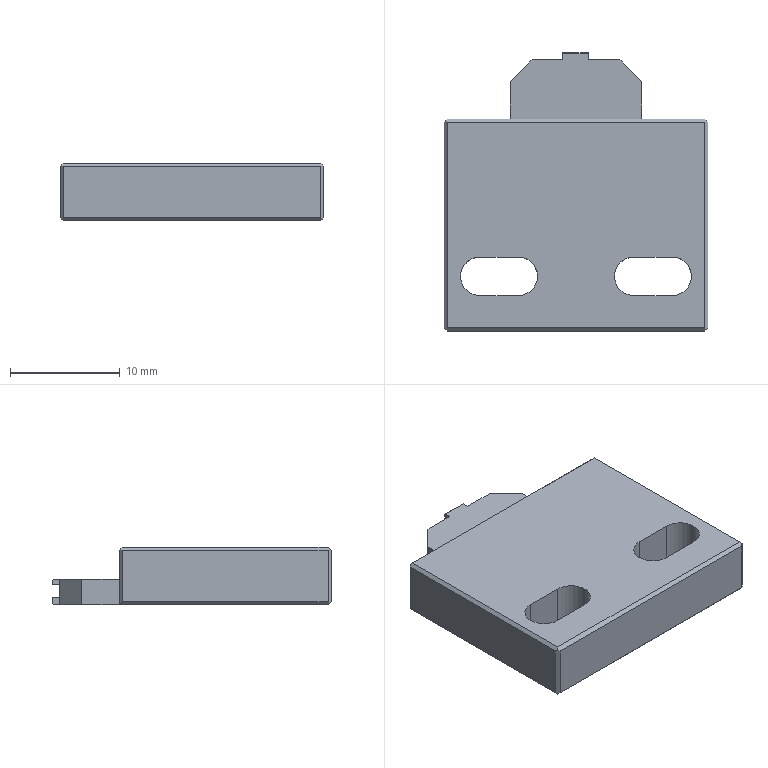Part | NX | 1 solid | 43 faces | box 24 x 25.342 x 5.25 mm | volume 2337 mm3 | plane 37 | cylinder 6 | commonest cylinder face diameters 3.5 x6
STEP:
#1=CARTESIAN_POINT('',(-1.2,-32.158,5.225));
#2=VERTEX_POINT('',#1);
#3=CARTESIAN_POINT('',(1.1,-32.158,5.225));
#4=VERTEX_POINT('',#3);
#5=CARTESIAN_POINT('',(-0.05,-32.158,5.225));
#6=DIRECTION('',(1.,0.,0.));
#7=VECTOR('',#6,1000.);
#8=LINE('',#5,#7);
#9=EDGE_CURVE('',#2,#4,#8,.T.);
#10=ORIENTED_EDGE('',*,*,#9,.T.);
#11=CARTESIAN_POINT('',(1.1,-32.158,4.822));
#12=VERTEX_POINT('',#11);
#13=CARTESIAN_POINT('',(1.1,-32.158,0.));
#14=DIRECTION('',(0.,0.,1.));
#15=VECTOR('',#14,1000.);
#16=LINE('',#13,#15);
#17=EDGE_CURVE('',#12,#4,#16,.T.);
#18=ORIENTED_EDGE('',*,*,#17,.F.);
#19=CARTESIAN_POINT('',(-1.2,-32.158,4.822));
#20=VERTEX_POINT('',#19);
#21=CARTESIAN_POINT('',(0.,-32.158,4.822));
#22=DIRECTION('',(-1.,0.,0.));
#23=VECTOR('',#22,1000.);
#24=LINE('',#21,#23);
#25=EDGE_CURVE('',#12,#20,#24,.T.);
#26=ORIENTED_EDGE('',*,*,#25,.T.);
#27=CARTESIAN_POINT('',(-1.2,-32.158,0.));
#28=DIRECTION('',(0.,0.,-1.));
#29=VECTOR('',#28,1000.);
#30=LINE('',#27,#29);
#31=EDGE_CURVE('',#2,#20,#30,.T.);
#32=ORIENTED_EDGE('',*,*,#31,.F.);
#33=EDGE_LOOP('',(#10,#18,#26,#32));
#34=FACE_BOUND('',#33,.T.);
#35=CARTESIAN_POINT('',(-4.2,-32.158,8.775));
#36=DIRECTION('',(0.,-1.,0.));
#37=DIRECTION('',(-1.,0.,0.));
#38=AXIS2_PLACEMENT_3D('',#35,#36,#37);
#39=PLANE('',#38);
#40=ADVANCED_FACE('',(#34),#39,.F.);
#41=ORIENTED_EDGE('',*,*,#9,.F.);
#42=CARTESIAN_POINT('',(-1.2,-32.258,5.325));
#43=VERTEX_POINT('',#42);
#44=CARTESIAN_POINT('',(-1.2,0.,-26.933));
#45=DIRECTION('',(0.,0.7071,-0.7071));
#46=VECTOR('',#45,1000.);
#47=LINE('',#44,#46);
#48=EDGE_CURVE('',#43,#2,#47,.T.);
#49=ORIENTED_EDGE('',*,*,#48,.F.);
#50=CARTESIAN_POINT('',(1.1,-32.258,5.325));
#51=VERTEX_POINT('',#50);
#52=CARTESIAN_POINT('',(-0.05,-32.258,5.325));
#53=DIRECTION('',(1.,0.,0.));
#54=VECTOR('',#53,1000.);
#55=LINE('',#52,#54);
#56=EDGE_CURVE('',#43,#51,#55,.T.);
#57=ORIENTED_EDGE('',*,*,#56,.T.);
#58=CARTESIAN_POINT('',(1.1,0.,-26.933));
#59=DIRECTION('',(0.,-0.7071,0.7071));
#60=VECTOR('',#59,1000.);
#61=LINE('',#58,#60);
#62=EDGE_CURVE('',#4,#51,#61,.T.);
#63=ORIENTED_EDGE('',*,*,#62,.F.);
#64=EDGE_LOOP('',(#41,#49,#57,#63));
#65=FACE_BOUND('',#64,.T.);
#66=CARTESIAN_POINT('',(-0.05,-32.208,5.275));
#67=DIRECTION('',(0.,0.7071,0.7071));
#68=DIRECTION('',(1.,0.,0.));
#69=AXIS2_PLACEMENT_3D('',#66,#67,#68);
#70=PLANE('',#69);
#71=ADVANCED_FACE('',(#65),#70,.T.);
#72=CARTESIAN_POINT('',(1.1,-32.158,3.1));
#73=VERTEX_POINT('',#72);
#74=CARTESIAN_POINT('',(-1.2,-32.158,3.1));
#75=VERTEX_POINT('',#74);
#76=CARTESIAN_POINT('',(-0.05,-32.158,3.1));
#77=DIRECTION('',(-1.,0.,0.));
#78=VECTOR('',#77,1000.);
#79=LINE('',#76,#78);
#80=EDGE_CURVE('',#73,#75,#79,.T.);
#81=ORIENTED_EDGE('',*,*,#80,.T.);
#82=CARTESIAN_POINT('',(-1.2,-32.158,3.7));
#83=VERTEX_POINT('',#82);
#84=CARTESIAN_POINT('',(-1.2,-32.158,0.));
#85=DIRECTION('',(0.,0.,-1.));
#86=VECTOR('',#85,1000.);
#87=LINE('',#84,#86);
#88=EDGE_CURVE('',#83,#75,#87,.T.);
#89=ORIENTED_EDGE('',*,*,#88,.F.);
#90=CARTESIAN_POINT('',(1.1,-32.158,3.7));
#91=VERTEX_POINT('',#90);
#92=CARTESIAN_POINT('',(0.,-32.158,3.7));
#93=DIRECTION('',(1.,0.,0.));
#94=VECTOR('',#93,1000.);
#95=LINE('',#92,#94);
#96=EDGE_CURVE('',#83,#91,#95,.T.);
#97=ORIENTED_EDGE('',*,*,#96,.T.);
#98=CARTESIAN_POINT('',(1.1,-32.158,0.));
#99=DIRECTION('',(0.,0.,1.));
#100=VECTOR('',#99,1000.);
#101=LINE('',#98,#100);
#102=EDGE_CURVE('',#73,#91,#101,.T.);
#103=ORIENTED_EDGE('',*,*,#102,.F.);
#104=EDGE_LOOP('',(#81,#89,#97,#103));
#105=FACE_BOUND('',#104,.T.);
#106=CARTESIAN_POINT('',(0.,-32.158,4.111));
#107=DIRECTION('',(0.,1.,0.));
#108=DIRECTION('',(1.,0.,0.));
#109=AXIS2_PLACEMENT_3D('',#106,#107,#108);
#110=PLANE('',#109);
#111=ADVANCED_FACE('',(#105),#110,.T.);
#112=ORIENTED_EDGE('',*,*,#80,.F.);
#113=CARTESIAN_POINT('',(1.1,-32.258,3.));
#114=VERTEX_POINT('',#113);
#115=CARTESIAN_POINT('',(1.1,0.,35.258));
#116=DIRECTION('',(0.,0.7071,0.7071));
#117=VECTOR('',#116,1000.);
#118=LINE('',#115,#117);
#119=EDGE_CURVE('',#114,#73,#118,.T.);
#120=ORIENTED_EDGE('',*,*,#119,.F.);
#121=CARTESIAN_POINT('',(-1.2,-32.258,3.));
#122=VERTEX_POINT('',#121);
#123=CARTESIAN_POINT('',(-0.05,-32.258,3.));
#124=DIRECTION('',(-1.,0.,0.));
#125=VECTOR('',#124,1000.);
#126=LINE('',#123,#125);
#127=EDGE_CURVE('',#114,#122,#126,.T.);
#128=ORIENTED_EDGE('',*,*,#127,.T.);
#129=CARTESIAN_POINT('',(-1.2,0.,35.258));
#130=DIRECTION('',(0.,-0.7071,-0.7071));
#131=VECTOR('',#130,1000.);
#132=LINE('',#129,#131);
#133=EDGE_CURVE('',#75,#122,#132,.T.);
#134=ORIENTED_EDGE('',*,*,#133,.F.);
#135=EDGE_LOOP('',(#112,#120,#128,#134));
#136=FACE_BOUND('',#135,.T.);
#137=CARTESIAN_POINT('',(-0.05,-32.208,3.05));
#138=DIRECTION('',(0.,0.7071,-0.7071));
#139=DIRECTION('',(-1.,0.,0.));
#140=AXIS2_PLACEMENT_3D('',#137,#138,#139);
#141=PLANE('',#140);
#142=ADVANCED_FACE('',(#136),#141,.T.);
#143=ORIENTED_EDGE('',*,*,#102,.T.);
#144=CARTESIAN_POINT('',(1.1,-32.815,3.7));
#145=VERTEX_POINT('',#144);
#146=CARTESIAN_POINT('',(1.1,0.,3.7));
#147=DIRECTION('',(0.,-1.,0.));
#148=VECTOR('',#147,1000.);
#149=LINE('',#146,#148);
#150=EDGE_CURVE('',#91,#145,#149,.T.);
#151=ORIENTED_EDGE('',*,*,#150,.T.);
#152=CARTESIAN_POINT('',(1.1,-32.815,3.));
#153=VERTEX_POINT('',#152);
#154=CARTESIAN_POINT('',(1.1,-32.815,0.));
#155=DIRECTION('',(0.,0.,1.));
#156=VECTOR('',#155,1000.);
#157=LINE('',#154,#156);
#158=EDGE_CURVE('',#153,#145,#157,.T.);
#159=ORIENTED_EDGE('',*,*,#158,.F.);
#160=CARTESIAN_POINT('',(1.1,0.,3.));
#161=DIRECTION('',(0.,1.,0.));
#162=VECTOR('',#161,1000.);
#163=LINE('',#160,#162);
#164=EDGE_CURVE('',#153,#114,#163,.T.);
#165=ORIENTED_EDGE('',*,*,#164,.T.);
#166=ORIENTED_EDGE('',*,*,#119,.T.);
#167=EDGE_LOOP('',(#143,#151,#159,#165,#166));
#168=FACE_BOUND('',#167,.T.);
#169=CARTESIAN_POINT('',(1.1,-33.565,2.475));
#170=DIRECTION('',(-1.,0.,0.));
#171=DIRECTION('',(0.,0.,1.));
#172=AXIS2_PLACEMENT_3D('',#169,#170,#171);
#173=PLANE('',#172);
#174=ADVANCED_FACE('',(#168),#173,.F.);
#175=ORIENTED_EDGE('',*,*,#150,.F.);
#176=ORIENTED_EDGE('',*,*,#96,.F.);
#177=CARTESIAN_POINT('',(-1.2,-32.815,3.7));
#178=VERTEX_POINT('',#177);
#179=CARTESIAN_POINT('',(-1.2,0.,3.7));
#180=DIRECTION('',(0.,1.,0.));
#181=VECTOR('',#180,1000.);
#182=LINE('',#179,#181);
#183=EDGE_CURVE('',#178,#83,#182,.T.);
#184=ORIENTED_EDGE('',*,*,#183,.F.);
#185=CARTESIAN_POINT('',(0.,-32.815,3.7));
#186=DIRECTION('',(-1.,0.,0.));
#187=VECTOR('',#186,1000.);
#188=LINE('',#185,#187);
#189=EDGE_CURVE('',#145,#178,#188,.T.);
#190=ORIENTED_EDGE('',*,*,#189,.F.);
#191=EDGE_LOOP('',(#175,#176,#184,#190));
#192=FACE_BOUND('',#191,.T.);
#193=CARTESIAN_POINT('',(6.,-34.,3.7));
#194=DIRECTION('',(0.,0.,1.));
#195=DIRECTION('',(0.,-1.,0.));
#196=AXIS2_PLACEMENT_3D('',#193,#194,#195);
#197=PLANE('',#196);
#198=ADVANCED_FACE('',(#192),#197,.T.);
#199=CARTESIAN_POINT('',(-4.,-32.815,5.325));
#200=VERTEX_POINT('',#199);
#201=CARTESIAN_POINT('',(-4.,-32.815,3.));
#202=VERTEX_POINT('',#201);
#203=CARTESIAN_POINT('',(-4.,-32.815,4.175));
#204=DIRECTION('',(0.,0.,-1.));
#205=VECTOR('',#204,1000.);
#206=LINE('',#203,#205);
#207=EDGE_CURVE('',#200,#202,#206,.T.);
#208=ORIENTED_EDGE('',*,*,#207,.F.);
#209=CARTESIAN_POINT('',(-1.2,-32.815,5.325));
#210=VERTEX_POINT('',#209);
#211=CARTESIAN_POINT('',(0.,-32.815,5.325));
#212=DIRECTION('',(1.,0.,0.));
#213=VECTOR('',#212,1000.);
#214=LINE('',#211,#213);
#215=EDGE_CURVE('',#200,#210,#214,.T.);
#216=ORIENTED_EDGE('',*,*,#215,.T.);
#217=CARTESIAN_POINT('',(-1.2,-32.815,4.822));
#218=VERTEX_POINT('',#217);
#219=CARTESIAN_POINT('',(-1.2,-32.815,0.));
#220=DIRECTION('',(0.,0.,-1.));
#221=VECTOR('',#220,1000.);
#222=LINE('',#219,#221);
#223=EDGE_CURVE('',#210,#218,#222,.T.);
#224=ORIENTED_EDGE('',*,*,#223,.T.);
#225=CARTESIAN_POINT('',(1.1,-32.815,4.822));
#226=VERTEX_POINT('',#225);
#227=CARTESIAN_POINT('',(0.,-32.815,4.822));
#228=DIRECTION('',(1.,0.,0.));
#229=VECTOR('',#228,1000.);
#230=LINE('',#227,#229);
#231=EDGE_CURVE('',#218,#226,#230,.T.);
#232=ORIENTED_EDGE('',*,*,#231,.T.);
#233=CARTESIAN_POINT('',(1.1,-32.815,5.325));
#234=VERTEX_POINT('',#233);
#235=CARTESIAN_POINT('',(1.1,-32.815,0.));
#236=DIRECTION('',(0.,0.,-1.));
#237=VECTOR('',#236,1000.);
#238=LINE('',#235,#237);
#239=EDGE_CURVE('',#234,#226,#238,.T.);
#240=ORIENTED_EDGE('',*,*,#239,.F.);
#241=CARTESIAN_POINT('',(4.,-32.815,5.325));
#242=VERTEX_POINT('',#241);
#243=CARTESIAN_POINT('',(0.,-32.815,5.325));
#244=DIRECTION('',(1.,0.,0.));
#245=VECTOR('',#244,1000.);
#246=LINE('',#243,#245);
#247=EDGE_CURVE('',#234,#242,#246,.T.);
#248=ORIENTED_EDGE('',*,*,#247,.T.);
#249=CARTESIAN_POINT('',(4.,-32.815,3.));
#250=VERTEX_POINT('',#249);
#251=CARTESIAN_POINT('',(4.,-32.815,4.175));
#252=DIRECTION('',(0.,0.,1.));
#253=VECTOR('',#252,1000.);
#254=LINE('',#251,#253);
#255=EDGE_CURVE('',#250,#242,#254,.T.);
#256=ORIENTED_EDGE('',*,*,#255,.F.);
#257=CARTESIAN_POINT('',(0.,-32.815,3.));
#258=DIRECTION('',(-1.,0.,0.));
#259=VECTOR('',#258,1000.);
#260=LINE('',#257,#259);
#261=EDGE_CURVE('',#250,#153,#260,.T.);
#262=ORIENTED_EDGE('',*,*,#261,.T.);
#263=ORIENTED_EDGE('',*,*,#158,.T.);
#264=ORIENTED_EDGE('',*,*,#189,.T.);
#265=CARTESIAN_POINT('',(-1.2,-32.815,3.));
#266=VERTEX_POINT('',#265);
#267=CARTESIAN_POINT('',(-1.2,-32.815,0.));
#268=DIRECTION('',(0.,0.,-1.));
#269=VECTOR('',#268,1000.);
#270=LINE('',#267,#269);
#271=EDGE_CURVE('',#178,#266,#270,.T.);
#272=ORIENTED_EDGE('',*,*,#271,.T.);
#273=CARTESIAN_POINT('',(0.,-32.815,3.));
#274=DIRECTION('',(-1.,0.,0.));
#275=VECTOR('',#274,1000.);
#276=LINE('',#273,#275);
#277=EDGE_CURVE('',#266,#202,#276,.T.);
#278=ORIENTED_EDGE('',*,*,#277,.T.);
#279=EDGE_LOOP('',(#208,#216,#224,#232,#240,#248,#256,#262,#263,#264,#272,#278));
#280=FACE_BOUND('',#279,.T.);
#281=CARTESIAN_POINT('',(6.,-32.815,2.475));
#282=DIRECTION('',(0.,-1.,0.));
#283=DIRECTION('',(0.,0.,-1.));
#284=AXIS2_PLACEMENT_3D('',#281,#282,#283);
#285=PLANE('',#284);
#286=ADVANCED_FACE('',(#280),#285,.F.);
#287=CARTESIAN_POINT('',(11.7,-38.2,3.));
#288=VERTEX_POINT('',#287);
#289=CARTESIAN_POINT('',(11.7,-57.2,3.));
#290=VERTEX_POINT('',#289);
#291=CARTESIAN_POINT('',(11.7,-47.85,3.));
#292=DIRECTION('',(0.,-1.,0.));
#293=VECTOR('',#292,1000.);
#294=LINE('',#291,#293);
#295=EDGE_CURVE('',#288,#290,#294,.T.);
#296=ORIENTED_EDGE('',*,*,#295,.T.);
#297=CARTESIAN_POINT('',(-11.7,-57.2,3.));
#298=VERTEX_POINT('',#297);
#299=CARTESIAN_POINT('',(0.,-57.2,3.));
#300=DIRECTION('',(1.,0.,0.));
#301=VECTOR('',#300,1000.);
#302=LINE('',#299,#301);
#303=EDGE_CURVE('',#298,#290,#302,.T.);
#304=ORIENTED_EDGE('',*,*,#303,.F.);
#305=CARTESIAN_POINT('',(-11.7,-38.2,3.));
#306=VERTEX_POINT('',#305);
#307=CARTESIAN_POINT('',(-11.7,-47.85,3.));
#308=DIRECTION('',(0.,-1.,0.));
#309=VECTOR('',#308,1000.);
#310=LINE('',#307,#309);
#311=EDGE_CURVE('',#306,#298,#310,.T.);
#312=ORIENTED_EDGE('',*,*,#311,.F.);
#313=CARTESIAN_POINT('',(-6.,-38.2,3.));
#314=VERTEX_POINT('',#313);
#315=CARTESIAN_POINT('',(0.,-38.2,3.));
#316=DIRECTION('',(-1.,0.,0.));
#317=VECTOR('',#316,1000.);
#318=LINE('',#315,#317);
#319=EDGE_CURVE('',#314,#306,#318,.T.);
#320=ORIENTED_EDGE('',*,*,#319,.F.);
#321=CARTESIAN_POINT('',(-6.,-34.815,3.));
#322=VERTEX_POINT('',#321);
#323=CARTESIAN_POINT('',(-6.,-33.565,3.));
#324=DIRECTION('',(0.,1.,0.));
#325=VECTOR('',#324,1000.);
#326=LINE('',#323,#325);
#327=EDGE_CURVE('',#314,#322,#326,.T.);
#328=ORIENTED_EDGE('',*,*,#327,.T.);
#329=CARTESIAN_POINT('',(28.815,0.,3.));
#330=DIRECTION('',(0.7071,0.7071,0.));
#331=VECTOR('',#330,1000.);
#332=LINE('',#329,#331);
#333=EDGE_CURVE('',#322,#202,#332,.T.);
#334=ORIENTED_EDGE('',*,*,#333,.T.);
#335=ORIENTED_EDGE('',*,*,#277,.F.);
#336=CARTESIAN_POINT('',(-1.2,0.,3.));
#337=DIRECTION('',(0.,-1.,0.));
#338=VECTOR('',#337,1000.);
#339=LINE('',#336,#338);
#340=EDGE_CURVE('',#122,#266,#339,.T.);
#341=ORIENTED_EDGE('',*,*,#340,.F.);
#342=ORIENTED_EDGE('',*,*,#127,.F.);
#343=ORIENTED_EDGE('',*,*,#164,.F.);
#344=ORIENTED_EDGE('',*,*,#261,.F.);
#345=CARTESIAN_POINT('',(6.,-34.815,3.));
#346=VERTEX_POINT('',#345);
#347=CARTESIAN_POINT('',(-28.815,0.,3.));
#348=DIRECTION('',(-0.7071,0.7071,0.));
#349=VECTOR('',#348,1000.);
#350=LINE('',#347,#349);
#351=EDGE_CURVE('',#346,#250,#350,.T.);
#352=ORIENTED_EDGE('',*,*,#351,.F.);
#353=CARTESIAN_POINT('',(6.,-38.2,3.));
#354=VERTEX_POINT('',#353);
#355=CARTESIAN_POINT('',(6.,0.,3.));
#356=DIRECTION('',(0.,1.,0.));
#357=VECTOR('',#356,1000.);
#358=LINE('',#355,#357);
#359=EDGE_CURVE('',#354,#346,#358,.T.);
#360=ORIENTED_EDGE('',*,*,#359,.F.);
#361=CARTESIAN_POINT('',(0.,-38.2,3.));
#362=DIRECTION('',(-1.,0.,0.));
#363=VECTOR('',#362,1000.);
#364=LINE('',#361,#363);
#365=EDGE_CURVE('',#288,#354,#364,.T.);
#366=ORIENTED_EDGE('',*,*,#365,.F.);
#367=EDGE_LOOP('',(#296,#304,#312,#320,#328,#334,#335,#341,#342,#343,#344,#352,#360,#366));
#368=FACE_BOUND('',#367,.T.);
#369=CARTESIAN_POINT('',(-5.25,-54.25,3.));
#370=VERTEX_POINT('',#369);
#371=CARTESIAN_POINT('',(-8.75,-54.25,3.));
#372=VERTEX_POINT('',#371);
#373=CARTESIAN_POINT('',(0.,-54.25,3.));
#374=DIRECTION('',(-1.,0.,0.));
#375=VECTOR('',#374,1000.);
#376=LINE('',#373,#375);
#377=EDGE_CURVE('',#370,#372,#376,.T.);
#378=ORIENTED_EDGE('',*,*,#377,.F.);
#379=CARTESIAN_POINT('',(-3.5,-52.5,3.));
#380=VERTEX_POINT('',#379);
#381=CARTESIAN_POINT('',(-5.25,-52.5,3.));
#382=DIRECTION('',(0.,0.,1.));
#383=DIRECTION('',(1.,0.,0.));
#384=AXIS2_PLACEMENT_3D('',#381,#382,#383);
#385=CIRCLE('',#384,1.75);
#386=EDGE_CURVE('',#370,#380,#385,.T.);
#387=ORIENTED_EDGE('',*,*,#386,.T.);
#388=CARTESIAN_POINT('',(-5.25,-50.75,3.));
#389=VERTEX_POINT('',#388);
#390=CARTESIAN_POINT('',(-5.25,-52.5,3.));
#391=DIRECTION('',(0.,0.,1.));
#392=DIRECTION('',(1.,0.,0.));
#393=AXIS2_PLACEMENT_3D('',#390,#391,#392);
#394=CIRCLE('',#393,1.75);
#395=EDGE_CURVE('',#380,#389,#394,.T.);
#396=ORIENTED_EDGE('',*,*,#395,.T.);
#397=CARTESIAN_POINT('',(-8.75,-50.75,3.));
#398=VERTEX_POINT('',#397);
#399=CARTESIAN_POINT('',(0.,-50.75,3.));
#400=DIRECTION('',(1.,0.,0.));
#401=VECTOR('',#400,1000.);
#402=LINE('',#399,#401);
#403=EDGE_CURVE('',#398,#389,#402,.T.);
#404=ORIENTED_EDGE('',*,*,#403,.F.);
#405=CARTESIAN_POINT('',(-8.75,-52.5,3.));
#406=DIRECTION('',(0.,0.,1.));
#407=DIRECTION('',(1.,0.,0.));
#408=AXIS2_PLACEMENT_3D('',#405,#406,#407);
#409=CIRCLE('',#408,1.75);
#410=EDGE_CURVE('',#398,#372,#409,.T.);
#411=ORIENTED_EDGE('',*,*,#410,.T.);
#412=EDGE_LOOP('',(#378,#387,#396,#404,#411));
#413=FACE_BOUND('',#412,.T.);
#414=CARTESIAN_POINT('',(8.75,-54.25,3.));
#415=VERTEX_POINT('',#414);
#416=CARTESIAN_POINT('',(5.25,-54.25,3.));
#417=VERTEX_POINT('',#416);
#418=CARTESIAN_POINT('',(0.,-54.25,3.));
#419=DIRECTION('',(-1.,0.,0.));
#420=VECTOR('',#419,1000.);
#421=LINE('',#418,#420);
#422=EDGE_CURVE('',#415,#417,#421,.T.);
#423=ORIENTED_EDGE('',*,*,#422,.F.);
#424=CARTESIAN_POINT('',(10.5,-52.5,3.));
#425=VERTEX_POINT('',#424);
#426=CARTESIAN_POINT('',(8.75,-52.5,3.));
#427=DIRECTION('',(0.,0.,1.));
#428=DIRECTION('',(1.,0.,0.));
#429=AXIS2_PLACEMENT_3D('',#426,#427,#428);
#430=CIRCLE('',#429,1.75);
#431=EDGE_CURVE('',#415,#425,#430,.T.);
#432=ORIENTED_EDGE('',*,*,#431,.T.);
#433=CARTESIAN_POINT('',(8.75,-50.75,3.));
#434=VERTEX_POINT('',#433);
#435=CARTESIAN_POINT('',(8.75,-52.5,3.));
#436=DIRECTION('',(0.,0.,1.));
#437=DIRECTION('',(1.,0.,0.));
#438=AXIS2_PLACEMENT_3D('',#435,#436,#437);
#439=CIRCLE('',#438,1.75);
#440=EDGE_CURVE('',#425,#434,#439,.T.);
#441=ORIENTED_EDGE('',*,*,#440,.T.);
#442=CARTESIAN_POINT('',(5.25,-50.75,3.));
#443=VERTEX_POINT('',#442);
#444=CARTESIAN_POINT('',(0.,-50.75,3.));
#445=DIRECTION('',(1.,0.,0.));
#446=VECTOR('',#445,1000.);
#447=LINE('',#444,#446);
#448=EDGE_CURVE('',#443,#434,#447,.T.);
#449=ORIENTED_EDGE('',*,*,#448,.F.);
#450=CARTESIAN_POINT('',(5.25,-52.5,3.));
#451=DIRECTION('',(0.,0.,1.));
#452=DIRECTION('',(1.,0.,0.));
#453=AXIS2_PLACEMENT_3D('',#450,#451,#452);
#454=CIRCLE('',#453,1.75);
#455=EDGE_CURVE('',#443,#417,#454,.T.);
#456=ORIENTED_EDGE('',*,*,#455,.T.);
#457=EDGE_LOOP('',(#423,#432,#441,#449,#456));
#458=FACE_BOUND('',#457,.T.);
#459=CARTESIAN_POINT('',(1.4,-33.565,3.));
#460=DIRECTION('',(0.,0.,-1.));
#461=DIRECTION('',(-1.,0.,0.));
#462=AXIS2_PLACEMENT_3D('',#459,#460,#461);
#463=PLANE('',#462);
#464=ADVANCED_FACE('',(#368,#413,#458),#463,.T.);
#465=CARTESIAN_POINT('',(10.5,-52.5,8.25));
#466=VERTEX_POINT('',#465);
#467=CARTESIAN_POINT('',(10.5,-52.5,2.475));
#468=DIRECTION('',(0.,0.,1.));
#469=VECTOR('',#468,1000.);
#470=LINE('',#467,#469);
#471=EDGE_CURVE('',#425,#466,#470,.T.);
#472=ORIENTED_EDGE('',*,*,#471,.F.);
#473=ORIENTED_EDGE('',*,*,#431,.F.);
#474=CARTESIAN_POINT('',(8.75,-54.25,8.25));
#475=VERTEX_POINT('',#474);
#476=CARTESIAN_POINT('',(8.75,-54.25,2.475));
#477=DIRECTION('',(0.,0.,1.));
#478=VECTOR('',#477,1000.);
#479=LINE('',#476,#478);
#480=EDGE_CURVE('',#415,#475,#479,.T.);
#481=ORIENTED_EDGE('',*,*,#480,.T.);
#482=CARTESIAN_POINT('',(8.75,-52.5,8.25));
#483=DIRECTION('',(0.,0.,1.));
#484=DIRECTION('',(1.,0.,0.));
#485=AXIS2_PLACEMENT_3D('',#482,#483,#484);
#486=CIRCLE('',#485,1.75);
#487=EDGE_CURVE('',#475,#466,#486,.T.);
#488=ORIENTED_EDGE('',*,*,#487,.T.);
#489=EDGE_LOOP('',(#472,#473,#481,#488));
#490=FACE_BOUND('',#489,.T.);
#491=CARTESIAN_POINT('',(8.75,-52.5,2.475));
#492=DIRECTION('',(0.,0.,1.));
#493=DIRECTION('',(1.,0.,0.));
#494=AXIS2_PLACEMENT_3D('',#491,#492,#493);
#495=CYLINDRICAL_SURFACE('',#494,1.75);
#496=ADVANCED_FACE('',(#490),#495,.F.);
#497=CARTESIAN_POINT('',(8.75,-50.75,8.25));
#498=VERTEX_POINT('',#497);
#499=CARTESIAN_POINT('',(5.25,-50.75,8.25));
#500=VERTEX_POINT('',#499);
#501=CARTESIAN_POINT('',(0.,-50.75,8.25));
#502=DIRECTION('',(-1.,0.,0.));
#503=VECTOR('',#502,1000.);
#504=LINE('',#501,#503);
#505=EDGE_CURVE('',#498,#500,#504,.T.);
#506=ORIENTED_EDGE('',*,*,#505,.T.);
#507=CARTESIAN_POINT('',(5.25,-50.75,2.475));
#508=DIRECTION('',(0.,0.,1.));
#509=VECTOR('',#508,1000.);
#510=LINE('',#507,#509);
#511=EDGE_CURVE('',#443,#500,#510,.T.);
#512=ORIENTED_EDGE('',*,*,#511,.F.);
#513=ORIENTED_EDGE('',*,*,#448,.T.);
#514=CARTESIAN_POINT('',(8.75,-50.75,2.475));
#515=DIRECTION('',(0.,0.,1.));
#516=VECTOR('',#515,1000.);
#517=LINE('',#514,#516);
#518=EDGE_CURVE('',#434,#498,#517,.T.);
#519=ORIENTED_EDGE('',*,*,#518,.T.);
#520=EDGE_LOOP('',(#506,#512,#513,#519));
#521=FACE_BOUND('',#520,.T.);
#522=CARTESIAN_POINT('',(5.25,-50.75,2.475));
#523=DIRECTION('',(0.,1.,0.));
#524=DIRECTION('',(1.,0.,0.));
#525=AXIS2_PLACEMENT_3D('',#522,#523,#524);
#526=PLANE('',#525);
#527=ADVANCED_FACE('',(#521),#526,.F.);
#528=ORIENTED_EDGE('',*,*,#422,.T.);
#529=CARTESIAN_POINT('',(5.25,-54.25,8.25));
#530=VERTEX_POINT('',#529);
#531=CARTESIAN_POINT('',(5.25,-54.25,2.475));
#532=DIRECTION('',(0.,0.,1.));
#533=VECTOR('',#532,1000.);
#534=LINE('',#531,#533);
#535=EDGE_CURVE('',#417,#530,#534,.T.);
#536=ORIENTED_EDGE('',*,*,#535,.T.);
#537=CARTESIAN_POINT('',(0.,-54.25,8.25));
#538=DIRECTION('',(1.,0.,0.));
#539=VECTOR('',#538,1000.);
#540=LINE('',#537,#539);
#541=EDGE_CURVE('',#530,#475,#540,.T.);
#542=ORIENTED_EDGE('',*,*,#541,.T.);
#543=ORIENTED_EDGE('',*,*,#480,.F.);
#544=EDGE_LOOP('',(#528,#536,#542,#543));
#545=FACE_BOUND('',#544,.T.);
#546=CARTESIAN_POINT('',(8.75,-54.25,2.475));
#547=DIRECTION('',(0.,-1.,0.));
#548=DIRECTION('',(0.,0.,-1.));
#549=AXIS2_PLACEMENT_3D('',#546,#547,#548);
#550=PLANE('',#549);
#551=ADVANCED_FACE('',(#545),#550,.F.);
#552=ORIENTED_EDGE('',*,*,#455,.F.);
#553=ORIENTED_EDGE('',*,*,#511,.T.);
#554=CARTESIAN_POINT('',(5.25,-52.5,8.25));
#555=DIRECTION('',(0.,0.,1.));
#556=DIRECTION('',(1.,0.,0.));
#557=AXIS2_PLACEMENT_3D('',#554,#555,#556);
#558=CIRCLE('',#557,1.75);
#559=EDGE_CURVE('',#500,#530,#558,.T.);
#560=ORIENTED_EDGE('',*,*,#559,.T.);
#561=ORIENTED_EDGE('',*,*,#535,.F.);
#562=EDGE_LOOP('',(#552,#553,#560,#561));
#563=FACE_BOUND('',#562,.T.);
#564=CARTESIAN_POINT('',(5.25,-52.5,2.475));
#565=DIRECTION('',(0.,0.,1.));
#566=DIRECTION('',(1.,0.,0.));
#567=AXIS2_PLACEMENT_3D('',#564,#565,#566);
#568=CYLINDRICAL_SURFACE('',#567,1.75);
#569=ADVANCED_FACE('',(#563),#568,.F.);
#570=ORIENTED_EDGE('',*,*,#207,.T.);
#571=ORIENTED_EDGE('',*,*,#333,.F.);
#572=CARTESIAN_POINT('',(-6.,-34.815,5.325));
#573=VERTEX_POINT('',#572);
#574=CARTESIAN_POINT('',(-6.,-34.815,4.175));
#575=DIRECTION('',(0.,0.,-1.));
#576=VECTOR('',#575,1000.);
#577=LINE('',#574,#576);
#578=EDGE_CURVE('',#573,#322,#577,.T.);
#579=ORIENTED_EDGE('',*,*,#578,.F.);
#580=CARTESIAN_POINT('',(28.815,0.,5.325));
#581=DIRECTION('',(0.7071,0.7071,0.));
#582=VECTOR('',#581,1000.);
#583=LINE('',#580,#582);
#584=EDGE_CURVE('',#573,#200,#583,.T.);
#585=ORIENTED_EDGE('',*,*,#584,.T.);
#586=EDGE_LOOP('',(#570,#571,#579,#585));
#587=FACE_BOUND('',#586,.T.);
#588=CARTESIAN_POINT('',(-5.,-33.815,4.175));
#589=DIRECTION('',(0.7071,-0.7071,0.));
#590=DIRECTION('',(0.,0.,-1.));
#591=AXIS2_PLACEMENT_3D('',#588,#589,#590);
#592=PLANE('',#591);
#593=ADVANCED_FACE('',(#587),#592,.F.);
#594=CARTESIAN_POINT('',(1.1,0.,5.325));
#595=DIRECTION('',(0.,-1.,0.));
#596=VECTOR('',#595,1000.);
#597=LINE('',#594,#596);
#598=EDGE_CURVE('',#51,#234,#597,.T.);
#599=ORIENTED_EDGE('',*,*,#598,.T.);
#600=ORIENTED_EDGE('',*,*,#239,.T.);
#601=CARTESIAN_POINT('',(1.1,-32.258,4.822));
#602=DIRECTION('',(0.,1.,0.));
#603=VECTOR('',#602,1000.);
#604=LINE('',#601,#603);
#605=EDGE_CURVE('',#226,#12,#604,.T.);
#606=ORIENTED_EDGE('',*,*,#605,.T.);
#607=ORIENTED_EDGE('',*,*,#17,.T.);
#608=ORIENTED_EDGE('',*,*,#62,.T.);
#609=EDGE_LOOP('',(#599,#600,#606,#607,#608));
#610=FACE_BOUND('',#609,.T.);
#611=CARTESIAN_POINT('',(1.1,-30.615,8.775));
#612=DIRECTION('',(-1.,0.,0.));
#613=DIRECTION('',(0.,0.,1.));
#614=AXIS2_PLACEMENT_3D('',#611,#612,#613);
#615=PLANE('',#614);
#616=ADVANCED_FACE('',(#610),#615,.F.);
#617=ORIENTED_EDGE('',*,*,#295,.F.);
#618=CARTESIAN_POINT('',(12.,-38.5,3.3));
#619=VERTEX_POINT('',#618);
#620=CARTESIAN_POINT('',(0.,-26.5,-8.7));
#621=DIRECTION('',(-0.5774,0.5774,-0.5774));
#622=VECTOR('',#621,1000.);
#623=LINE('',#620,#622);
#624=EDGE_CURVE('',#619,#288,#623,.T.);
#625=ORIENTED_EDGE('',*,*,#624,.F.);
#626=CARTESIAN_POINT('',(12.,-57.2,3.3));
#627=VERTEX_POINT('',#626);
#628=CARTESIAN_POINT('',(12.,-47.85,3.3));
#629=DIRECTION('',(0.,-1.,0.));
#630=VECTOR('',#629,1000.);
#631=LINE('',#628,#630);
#632=EDGE_CURVE('',#619,#627,#631,.T.);
#633=ORIENTED_EDGE('',*,*,#632,.T.);
#634=CARTESIAN_POINT('',(11.85,-57.35,3.15));
#635=VERTEX_POINT('',#634);
#636=CARTESIAN_POINT('',(0.,-69.2,-8.7));
#637=DIRECTION('',(-0.5774,-0.5774,-0.5774));
#638=VECTOR('',#637,1000.);
#639=LINE('',#636,#638);
#640=EDGE_CURVE('',#627,#635,#639,.T.);
#641=ORIENTED_EDGE('',*,*,#640,.T.);
#642=CARTESIAN_POINT('',(0.,-45.5,-8.7));
#643=DIRECTION('',(0.5774,-0.5774,0.5774));
#644=VECTOR('',#643,1000.);
#645=LINE('',#642,#644);
#646=EDGE_CURVE('',#290,#635,#645,.T.);
#647=ORIENTED_EDGE('',*,*,#646,.F.);
#648=EDGE_LOOP('',(#617,#625,#633,#641,#647));
#649=FACE_BOUND('',#648,.T.);
#650=CARTESIAN_POINT('',(11.85,-47.85,3.15));
#651=DIRECTION('',(0.7071,0.,-0.7071));
#652=DIRECTION('',(0.,-1.,0.));
#653=AXIS2_PLACEMENT_3D('',#650,#651,#652);
#654=PLANE('',#653);
#655=ADVANCED_FACE('',(#649),#654,.T.);
#656=CARTESIAN_POINT('',(-1.2,0.,4.822));
#657=DIRECTION('',(0.,-1.,0.));
#658=VECTOR('',#657,1000.);
#659=LINE('',#656,#658);
#660=EDGE_CURVE('',#20,#218,#659,.T.);
#661=ORIENTED_EDGE('',*,*,#660,.T.);
#662=ORIENTED_EDGE('',*,*,#223,.F.);
#663=CARTESIAN_POINT('',(-1.2,0.,5.325));
#664=DIRECTION('',(0.,1.,0.));
#665=VECTOR('',#664,1000.);
#666=LINE('',#663,#665);
#667=EDGE_CURVE('',#210,#43,#666,.T.);
#668=ORIENTED_EDGE('',*,*,#667,.T.);
#669=ORIENTED_EDGE('',*,*,#48,.T.);
#670=ORIENTED_EDGE('',*,*,#31,.T.);
#671=EDGE_LOOP('',(#661,#662,#668,#669,#670));
#672=FACE_BOUND('',#671,.T.);
#673=CARTESIAN_POINT('',(-1.2,-32.815,8.775));
#674=DIRECTION('',(1.,0.,0.));
#675=DIRECTION('',(0.,-1.,0.));
#676=AXIS2_PLACEMENT_3D('',#673,#674,#675);
#677=PLANE('',#676);
#678=ADVANCED_FACE('',(#672),#677,.F.);
#679=ORIENTED_EDGE('',*,*,#605,.F.);
#680=ORIENTED_EDGE('',*,*,#231,.F.);
#681=ORIENTED_EDGE('',*,*,#660,.F.);
#682=ORIENTED_EDGE('',*,*,#25,.F.);
#683=EDGE_LOOP('',(#679,#680,#681,#682));
#684=FACE_BOUND('',#683,.T.);
#685=CARTESIAN_POINT('',(-1.577,-32.815,4.822));
#686=DIRECTION('',(0.,0.,-1.));
#687=DIRECTION('',(-1.,0.,0.));
#688=AXIS2_PLACEMENT_3D('',#685,#686,#687);
#689=PLANE('',#688);
#690=ADVANCED_FACE('',(#684),#689,.T.);
#691=ORIENTED_EDGE('',*,*,#340,.T.);
#692=ORIENTED_EDGE('',*,*,#271,.F.);
#693=ORIENTED_EDGE('',*,*,#183,.T.);
#694=ORIENTED_EDGE('',*,*,#88,.T.);
#695=ORIENTED_EDGE('',*,*,#133,.T.);
#696=EDGE_LOOP('',(#691,#692,#693,#694,#695));
#697=FACE_BOUND('',#696,.T.);
#698=CARTESIAN_POINT('',(-1.2,-32.258,2.475));
#699=DIRECTION('',(1.,0.,0.));
#700=DIRECTION('',(0.,1.,0.));
#701=AXIS2_PLACEMENT_3D('',#698,#699,#700);
#702=PLANE('',#701);
#703=ADVANCED_FACE('',(#697),#702,.F.);
#704=CARTESIAN_POINT('',(-11.7,-57.5,3.3));
#705=VERTEX_POINT('',#704);
#706=CARTESIAN_POINT('',(11.7,-57.5,3.3));
#707=VERTEX_POINT('',#706);
#708=CARTESIAN_POINT('',(0.,-57.5,3.3));
#709=DIRECTION('',(1.,0.,0.));
#710=VECTOR('',#709,1000.);
#711=LINE('',#708,#710);
#712=EDGE_CURVE('',#705,#707,#711,.T.);
#713=ORIENTED_EDGE('',*,*,#712,.T.);
#714=CARTESIAN_POINT('',(11.7,-57.5,7.95));
#715=VERTEX_POINT('',#714);
#716=CARTESIAN_POINT('',(11.7,-57.5,0.));
#717=DIRECTION('',(0.,0.,1.));
#718=VECTOR('',#717,1000.);
#719=LINE('',#716,#718);
#720=EDGE_CURVE('',#707,#715,#719,.T.);
#721=ORIENTED_EDGE('',*,*,#720,.T.);
#722=CARTESIAN_POINT('',(-11.7,-57.5,7.95));
#723=VERTEX_POINT('',#722);
#724=CARTESIAN_POINT('',(0.,-57.5,7.95));
#725=DIRECTION('',(-1.,0.,0.));
#726=VECTOR('',#725,1000.);
#727=LINE('',#724,#726);
#728=EDGE_CURVE('',#715,#723,#727,.T.);
#729=ORIENTED_EDGE('',*,*,#728,.T.);
#730=CARTESIAN_POINT('',(-11.7,-57.5,0.));
#731=DIRECTION('',(0.,0.,-1.));
#732=VECTOR('',#731,1000.);
#733=LINE('',#730,#732);
#734=EDGE_CURVE('',#723,#705,#733,.T.);
#735=ORIENTED_EDGE('',*,*,#734,.T.);
#736=EDGE_LOOP('',(#713,#721,#729,#735));
#737=FACE_BOUND('',#736,.T.);
#738=CARTESIAN_POINT('',(-8.,-57.5,0.000000001));
#739=DIRECTION('',(0.,-1.,0.));
#740=DIRECTION('',(0.,0.,-1.));
#741=AXIS2_PLACEMENT_3D('',#738,#739,#740);
#742=PLANE('',#741);
#743=ADVANCED_FACE('',(#737),#742,.T.);
#744=CARTESIAN_POINT('',(-12.,-57.2,7.95));
#745=VERTEX_POINT('',#744);
#746=CARTESIAN_POINT('',(-12.,-57.2,3.3));
#747=VERTEX_POINT('',#746);
#748=CARTESIAN_POINT('',(-12.,-57.2,0.));
#749=DIRECTION('',(0.,0.,-1.));
#750=VECTOR('',#749,1000.);
#751=LINE('',#748,#750);
#752=EDGE_CURVE('',#745,#747,#751,.T.);
#753=ORIENTED_EDGE('',*,*,#752,.T.);
#754=CARTESIAN_POINT('',(-11.85,-57.35,3.15));
#755=VERTEX_POINT('',#754);
#756=CARTESIAN_POINT('',(0.,-69.2,-8.7));
#757=DIRECTION('',(-0.5774,0.5774,0.5774));
#758=VECTOR('',#757,1000.);
#759=LINE('',#756,#758);
#760=EDGE_CURVE('',#755,#747,#759,.T.);
#761=ORIENTED_EDGE('',*,*,#760,.F.);
#762=CARTESIAN_POINT('',(0.,-69.2,15.));
#763=DIRECTION('',(-0.5774,0.5774,-0.5774));
#764=VECTOR('',#763,1000.);
#765=LINE('',#762,#764);
#766=EDGE_CURVE('',#705,#755,#765,.T.);
#767=ORIENTED_EDGE('',*,*,#766,.F.);
#768=ORIENTED_EDGE('',*,*,#734,.F.);
#769=CARTESIAN_POINT('',(-11.85,-57.35,8.1));
#770=VERTEX_POINT('',#769);
#771=CARTESIAN_POINT('',(0.,-69.2,-3.75));
#772=DIRECTION('',(0.5774,-0.5774,-0.5774));
#773=VECTOR('',#772,1000.);
#774=LINE('',#771,#773);
#775=EDGE_CURVE('',#770,#723,#774,.T.);
#776=ORIENTED_EDGE('',*,*,#775,.F.);
#777=CARTESIAN_POINT('',(0.,-69.2,19.95));
#778=DIRECTION('',(0.5774,-0.5774,0.5774));
#779=VECTOR('',#778,1000.);
#780=LINE('',#777,#779);
#781=EDGE_CURVE('',#745,#770,#780,.T.);
#782=ORIENTED_EDGE('',*,*,#781,.F.);
#783=EDGE_LOOP('',(#753,#761,#767,#768,#776,#782));
#784=FACE_BOUND('',#783,.T.);
#785=CARTESIAN_POINT('',(-11.85,-57.35,5.625));
#786=DIRECTION('',(-0.7071,-0.7071,0.));
#787=DIRECTION('',(-0.7071,0.7071,0.));
#788=AXIS2_PLACEMENT_3D('',#785,#786,#787);
#789=PLANE('',#788);
#790=ADVANCED_FACE('',(#784),#789,.T.);
#791=CARTESIAN_POINT('',(-12.,-38.5,3.3));
#792=VERTEX_POINT('',#791);
#793=CARTESIAN_POINT('',(-12.,-47.85,3.3));
#794=DIRECTION('',(0.,-1.,0.));
#795=VECTOR('',#794,1000.);
#796=LINE('',#793,#795);
#797=EDGE_CURVE('',#792,#747,#796,.T.);
#798=ORIENTED_EDGE('',*,*,#797,.T.);
#799=ORIENTED_EDGE('',*,*,#752,.F.);
#800=CARTESIAN_POINT('',(-12.,-38.5,7.95));
#801=VERTEX_POINT('',#800);
#802=CARTESIAN_POINT('',(-12.,-47.85,7.95));
#803=DIRECTION('',(0.,1.,0.));
#804=VECTOR('',#803,1000.);
#805=LINE('',#802,#804);
#806=EDGE_CURVE('',#745,#801,#805,.T.);
#807=ORIENTED_EDGE('',*,*,#806,.T.);
#808=CARTESIAN_POINT('',(-12.,-38.5,0.));
#809=DIRECTION('',(0.,0.,1.));
#810=VECTOR('',#809,1000.);
#811=LINE('',#808,#810);
#812=EDGE_CURVE('',#792,#801,#811,.T.);
#813=ORIENTED_EDGE('',*,*,#812,.F.);
#814=EDGE_LOOP('',(#798,#799,#807,#813));
#815=FACE_BOUND('',#814,.T.);
#816=CARTESIAN_POINT('',(-12.,9.5,0.000000001));
#817=DIRECTION('',(-1.,0.,0.));
#818=DIRECTION('',(0.,0.,1.));
#819=AXIS2_PLACEMENT_3D('',#816,#817,#818);
#820=PLANE('',#819);
#821=ADVANCED_FACE('',(#815),#820,.T.);
#822=ORIENTED_EDGE('',*,*,#377,.T.);
#823=CARTESIAN_POINT('',(-8.75,-54.25,8.25));
#824=VERTEX_POINT('',#823);
#825=CARTESIAN_POINT('',(-8.75,-54.25,2.475));
#826=DIRECTION('',(0.,0.,1.));
#827=VECTOR('',#826,1000.);
#828=LINE('',#825,#827);
#829=EDGE_CURVE('',#372,#824,#828,.T.);
#830=ORIENTED_EDGE('',*,*,#829,.T.);
#831=CARTESIAN_POINT('',(-5.25,-54.25,8.25));
#832=VERTEX_POINT('',#831);
#833=CARTESIAN_POINT('',(0.,-54.25,8.25));
#834=DIRECTION('',(1.,0.,0.));
#835=VECTOR('',#834,1000.);
#836=LINE('',#833,#835);
#837=EDGE_CURVE('',#824,#832,#836,.T.);
#838=ORIENTED_EDGE('',*,*,#837,.T.);
#839=CARTESIAN_POINT('',(-5.25,-54.25,2.475));
#840=DIRECTION('',(0.,0.,1.));
#841=VECTOR('',#840,1000.);
#842=LINE('',#839,#841);
#843=EDGE_CURVE('',#370,#832,#842,.T.);
#844=ORIENTED_EDGE('',*,*,#843,.F.);
#845=EDGE_LOOP('',(#822,#830,#838,#844));
#846=FACE_BOUND('',#845,.T.);
#847=CARTESIAN_POINT('',(-5.25,-54.25,2.475));
#848=DIRECTION('',(0.,-1.,0.));
#849=DIRECTION('',(0.,0.,-1.));
#850=AXIS2_PLACEMENT_3D('',#847,#848,#849);
#851=PLANE('',#850);
#852=ADVANCED_FACE('',(#846),#851,.F.);
#853=ORIENTED_EDGE('',*,*,#720,.F.);
#854=CARTESIAN_POINT('',(0.,-69.2,15.));
#855=DIRECTION('',(-0.5774,-0.5774,0.5774));
#856=VECTOR('',#855,1000.);
#857=LINE('',#854,#856);
#858=EDGE_CURVE('',#635,#707,#857,.T.);
#859=ORIENTED_EDGE('',*,*,#858,.F.);
#860=ORIENTED_EDGE('',*,*,#640,.F.);
#861=CARTESIAN_POINT('',(12.,-57.2,7.95));
#862=VERTEX_POINT('',#861);
#863=CARTESIAN_POINT('',(12.,-57.2,0.));
#864=DIRECTION('',(0.,0.,1.));
#865=VECTOR('',#864,1000.);
#866=LINE('',#863,#865);
#867=EDGE_CURVE('',#627,#862,#866,.T.);
#868=ORIENTED_EDGE('',*,*,#867,.T.);
#869=CARTESIAN_POINT('',(11.85,-57.35,8.1));
#870=VERTEX_POINT('',#869);
#871=CARTESIAN_POINT('',(0.,-69.2,19.95));
#872=DIRECTION('',(-0.5774,-0.5774,0.5774));
#873=VECTOR('',#872,1000.);
#874=LINE('',#871,#873);
#875=EDGE_CURVE('',#862,#870,#874,.T.);
#876=ORIENTED_EDGE('',*,*,#875,.T.);
#877=CARTESIAN_POINT('',(0.,-69.2,-3.75));
#878=DIRECTION('',(-0.5774,-0.5774,-0.5774));
#879=VECTOR('',#878,1000.);
#880=LINE('',#877,#879);
#881=EDGE_CURVE('',#870,#715,#880,.T.);
#882=ORIENTED_EDGE('',*,*,#881,.T.);
#883=EDGE_LOOP('',(#853,#859,#860,#868,#876,#882));
#884=FACE_BOUND('',#883,.T.);
#885=CARTESIAN_POINT('',(11.85,-57.35,5.625));
#886=DIRECTION('',(0.7071,-0.7071,0.));
#887=DIRECTION('',(0.,0.,-1.));
#888=AXIS2_PLACEMENT_3D('',#885,#886,#887);
#889=PLANE('',#888);
#890=ADVANCED_FACE('',(#884),#889,.T.);
#891=CARTESIAN_POINT('',(11.7,-38.5,8.25));
#892=VERTEX_POINT('',#891);
#893=CARTESIAN_POINT('',(-11.7,-38.5,8.25));
#894=VERTEX_POINT('',#893);
#895=CARTESIAN_POINT('',(0.,-38.5,8.25));
#896=DIRECTION('',(-1.,0.,0.));
#897=VECTOR('',#896,1000.);
#898=LINE('',#895,#897);
#899=EDGE_CURVE('',#892,#894,#898,.T.);
#900=ORIENTED_EDGE('',*,*,#899,.F.);
#901=CARTESIAN_POINT('',(11.85,-38.35,8.1));
#902=VERTEX_POINT('',#901);
#903=CARTESIAN_POINT('',(0.,-50.2,19.95));
#904=DIRECTION('',(-0.5774,-0.5774,0.5774));
#905=VECTOR('',#904,1000.);
#906=LINE('',#903,#905);
#907=EDGE_CURVE('',#902,#892,#906,.T.);
#908=ORIENTED_EDGE('',*,*,#907,.F.);
#909=CARTESIAN_POINT('',(11.7,-38.2,7.95));
#910=VERTEX_POINT('',#909);
#911=CARTESIAN_POINT('',(0.,-26.5,-3.75));
#912=DIRECTION('',(0.5774,-0.5774,0.5774));
#913=VECTOR('',#912,1000.);
#914=LINE('',#911,#913);
#915=EDGE_CURVE('',#910,#902,#914,.T.);
#916=ORIENTED_EDGE('',*,*,#915,.F.);
#917=CARTESIAN_POINT('',(-11.7,-38.2,7.95));
#918=VERTEX_POINT('',#917);
#919=CARTESIAN_POINT('',(0.,-38.2,7.95));
#920=DIRECTION('',(-1.,0.,0.));
#921=VECTOR('',#920,1000.);
#922=LINE('',#919,#921);
#923=EDGE_CURVE('',#910,#918,#922,.T.);
#924=ORIENTED_EDGE('',*,*,#923,.T.);
#925=CARTESIAN_POINT('',(-11.85,-38.35,8.1));
#926=VERTEX_POINT('',#925);
#927=CARTESIAN_POINT('',(0.,-26.5,-3.75));
#928=DIRECTION('',(0.5774,0.5774,-0.5774));
#929=VECTOR('',#928,1000.);
#930=LINE('',#927,#929);
#931=EDGE_CURVE('',#926,#918,#930,.T.);
#932=ORIENTED_EDGE('',*,*,#931,.F.);
#933=CARTESIAN_POINT('',(0.,-50.2,19.95));
#934=DIRECTION('',(0.5774,-0.5774,0.5774));
#935=VECTOR('',#934,1000.);
#936=LINE('',#933,#935);
#937=EDGE_CURVE('',#926,#894,#936,.T.);
#938=ORIENTED_EDGE('',*,*,#937,.T.);
#939=EDGE_LOOP('',(#900,#908,#916,#924,#932,#938));
#940=FACE_BOUND('',#939,.T.);
#941=CARTESIAN_POINT('',(0.,-38.35,8.1));
#942=DIRECTION('',(0.,0.7071,0.7071));
#943=DIRECTION('',(1.,0.,0.));
#944=AXIS2_PLACEMENT_3D('',#941,#942,#943);
#945=PLANE('',#944);
#946=ADVANCED_FACE('',(#940),#945,.T.);
#947=ORIENTED_EDGE('',*,*,#899,.T.);
#948=CARTESIAN_POINT('',(-11.7,-57.2,8.25));
#949=VERTEX_POINT('',#948);
#950=CARTESIAN_POINT('',(-11.7,-47.85,8.25));
#951=DIRECTION('',(0.,1.,0.));
#952=VECTOR('',#951,1000.);
#953=LINE('',#950,#952);
#954=EDGE_CURVE('',#949,#894,#953,.T.);
#955=ORIENTED_EDGE('',*,*,#954,.F.);
#956=CARTESIAN_POINT('',(11.7,-57.2,8.25));
#957=VERTEX_POINT('',#956);
#958=CARTESIAN_POINT('',(0.,-57.2,8.25));
#959=DIRECTION('',(-1.,0.,0.));
#960=VECTOR('',#959,1000.);
#961=LINE('',#958,#960);
#962=EDGE_CURVE('',#957,#949,#961,.T.);
#963=ORIENTED_EDGE('',*,*,#962,.F.);
#964=CARTESIAN_POINT('',(11.7,-47.85,8.25));
#965=DIRECTION('',(0.,-1.,0.));
#966=VECTOR('',#965,1000.);
#967=LINE('',#964,#966);
#968=EDGE_CURVE('',#892,#957,#967,.T.);
#969=ORIENTED_EDGE('',*,*,#968,.F.);
#970=EDGE_LOOP('',(#947,#955,#963,#969));
#971=FACE_BOUND('',#970,.T.);
#972=CARTESIAN_POINT('',(-5.25,-50.75,8.25));
#973=VERTEX_POINT('',#972);
#974=CARTESIAN_POINT('',(-8.75,-50.75,8.25));
#975=VERTEX_POINT('',#974);
#976=CARTESIAN_POINT('',(0.,-50.75,8.25));
#977=DIRECTION('',(-1.,0.,0.));
#978=VECTOR('',#977,1000.);
#979=LINE('',#976,#978);
#980=EDGE_CURVE('',#973,#975,#979,.T.);
#981=ORIENTED_EDGE('',*,*,#980,.F.);
#982=CARTESIAN_POINT('',(-3.5,-52.5,8.25));
#983=VERTEX_POINT('',#982);
#984=CARTESIAN_POINT('',(-5.25,-52.5,8.25));
#985=DIRECTION('',(0.,0.,1.));
#986=DIRECTION('',(1.,0.,0.));
#987=AXIS2_PLACEMENT_3D('',#984,#985,#986);
#988=CIRCLE('',#987,1.75);
#989=EDGE_CURVE('',#983,#973,#988,.T.);
#990=ORIENTED_EDGE('',*,*,#989,.F.);
#991=CARTESIAN_POINT('',(-5.25,-52.5,8.25));
#992=DIRECTION('',(0.,0.,1.));
#993=DIRECTION('',(1.,0.,0.));
#994=AXIS2_PLACEMENT_3D('',#991,#992,#993);
#995=CIRCLE('',#994,1.75);
#996=EDGE_CURVE('',#832,#983,#995,.T.);
#997=ORIENTED_EDGE('',*,*,#996,.F.);
#998=ORIENTED_EDGE('',*,*,#837,.F.);
#999=CARTESIAN_POINT('',(-8.75,-52.5,8.25));
#1000=DIRECTION('',(0.,0.,1.));
#1001=DIRECTION('',(1.,0.,0.));
#1002=AXIS2_PLACEMENT_3D('',#999,#1000,#1001);
#1003=CIRCLE('',#1002,1.75);
#1004=EDGE_CURVE('',#975,#824,#1003,.T.);
#1005=ORIENTED_EDGE('',*,*,#1004,.F.);
#1006=EDGE_LOOP('',(#981,#990,#997,#998,#1005));
#1007=FACE_BOUND('',#1006,.T.);
#1008=ORIENTED_EDGE('',*,*,#505,.F.);
#1009=CARTESIAN_POINT('',(8.75,-52.5,8.25));
#1010=DIRECTION('',(0.,0.,1.));
#1011=DIRECTION('',(1.,0.,0.));
#1012=AXIS2_PLACEMENT_3D('',#1009,#1010,#1011);
#1013=CIRCLE('',#1012,1.75);
#1014=EDGE_CURVE('',#466,#498,#1013,.T.);
#1015=ORIENTED_EDGE('',*,*,#1014,.F.);
#1016=ORIENTED_EDGE('',*,*,#487,.F.);
#1017=ORIENTED_EDGE('',*,*,#541,.F.);
#1018=ORIENTED_EDGE('',*,*,#559,.F.);
#1019=EDGE_LOOP('',(#1008,#1015,#1016,#1017,#1018));
#1020=FACE_BOUND('',#1019,.T.);
#1021=CARTESIAN_POINT('',(0.,-38.,8.25));
#1022=DIRECTION('',(0.,0.,1.));
#1023=DIRECTION('',(1.,0.,0.));
#1024=AXIS2_PLACEMENT_3D('',#1021,#1022,#1023);
#1025=PLANE('',#1024);
#1026=ADVANCED_FACE('',(#971,#1007,#1020),#1025,.T.);
#1027=ORIENTED_EDGE('',*,*,#632,.F.);
#1028=CARTESIAN_POINT('',(12.,-38.5,7.95));
#1029=VERTEX_POINT('',#1028);
#1030=CARTESIAN_POINT('',(12.,-38.5,0.));
#1031=DIRECTION('',(0.,0.,-1.));
#1032=VECTOR('',#1031,1000.);
#1033=LINE('',#1030,#1032);
#1034=EDGE_CURVE('',#1029,#619,#1033,.T.);
#1035=ORIENTED_EDGE('',*,*,#1034,.F.);
#1036=CARTESIAN_POINT('',(12.,-47.85,7.95));
#1037=DIRECTION('',(0.,-1.,0.));
#1038=VECTOR('',#1037,1000.);
#1039=LINE('',#1036,#1038);
#1040=EDGE_CURVE('',#1029,#862,#1039,.T.);
#1041=ORIENTED_EDGE('',*,*,#1040,.T.);
#1042=ORIENTED_EDGE('',*,*,#867,.F.);
#1043=EDGE_LOOP('',(#1027,#1035,#1041,#1042));
#1044=FACE_BOUND('',#1043,.T.);
#1045=CARTESIAN_POINT('',(12.,-38.,0.000000001));
#1046=DIRECTION('',(1.,0.,0.));
#1047=DIRECTION('',(0.,1.,0.));
#1048=AXIS2_PLACEMENT_3D('',#1045,#1046,#1047);
#1049=PLANE('',#1048);
#1050=ADVANCED_FACE('',(#1044),#1049,.T.);
#1051=CARTESIAN_POINT('',(6.,-38.2,5.325));
#1052=VERTEX_POINT('',#1051);
#1053=CARTESIAN_POINT('',(6.,-38.2,0.));
#1054=DIRECTION('',(0.,0.,1.));
#1055=VECTOR('',#1054,1000.);
#1056=LINE('',#1053,#1055);
#1057=EDGE_CURVE('',#354,#1052,#1056,.T.);
#1058=ORIENTED_EDGE('',*,*,#1057,.F.);
#1059=ORIENTED_EDGE('',*,*,#359,.T.);
#1060=CARTESIAN_POINT('',(6.,-34.815,5.325));
#1061=VERTEX_POINT('',#1060);
#1062=CARTESIAN_POINT('',(6.,-34.815,4.175));
#1063=DIRECTION('',(0.,0.,1.));
#1064=VECTOR('',#1063,1000.);
#1065=LINE('',#1062,#1064);
#1066=EDGE_CURVE('',#346,#1061,#1065,.T.);
#1067=ORIENTED_EDGE('',*,*,#1066,.T.);
#1068=CARTESIAN_POINT('',(6.,0.,5.325));
#1069=DIRECTION('',(0.,-1.,0.));
#1070=VECTOR('',#1069,1000.);
#1071=LINE('',#1068,#1070);
#1072=EDGE_CURVE('',#1061,#1052,#1071,.T.);
#1073=ORIENTED_EDGE('',*,*,#1072,.T.);
#1074=EDGE_LOOP('',(#1058,#1059,#1067,#1073));
#1075=FACE_BOUND('',#1074,.T.);
#1076=CARTESIAN_POINT('',(6.,-40.5,2.5));
#1077=DIRECTION('',(-1.,0.,0.));
#1078=DIRECTION('',(0.,0.,1.));
#1079=AXIS2_PLACEMENT_3D('',#1076,#1077,#1078);
#1080=PLANE('',#1079);
#1081=ADVANCED_FACE('',(#1075),#1080,.F.);
#1082=ORIENTED_EDGE('',*,*,#980,.T.);
#1083=CARTESIAN_POINT('',(-8.75,-50.75,2.475));
#1084=DIRECTION('',(0.,0.,1.));
#1085=VECTOR('',#1084,1000.);
#1086=LINE('',#1083,#1085);
#1087=EDGE_CURVE('',#398,#975,#1086,.T.);
#1088=ORIENTED_EDGE('',*,*,#1087,.F.);
#1089=ORIENTED_EDGE('',*,*,#403,.T.);
#1090=CARTESIAN_POINT('',(-5.25,-50.75,2.475));
#1091=DIRECTION('',(0.,0.,1.));
#1092=VECTOR('',#1091,1000.);
#1093=LINE('',#1090,#1092);
#1094=EDGE_CURVE('',#389,#973,#1093,.T.);
#1095=ORIENTED_EDGE('',*,*,#1094,.T.);
#1096=EDGE_LOOP('',(#1082,#1088,#1089,#1095));
#1097=FACE_BOUND('',#1096,.T.);
#1098=CARTESIAN_POINT('',(-8.75,-50.75,2.475));
#1099=DIRECTION('',(0.,1.,0.));
#1100=DIRECTION('',(1.,0.,0.));
#1101=AXIS2_PLACEMENT_3D('',#1098,#1099,#1100);
#1102=PLANE('',#1101);
#1103=ADVANCED_FACE('',(#1097),#1102,.F.);
#1104=ORIENTED_EDGE('',*,*,#923,.F.);
#1105=CARTESIAN_POINT('',(11.7,-38.2,5.625));
#1106=DIRECTION('',(0.,0.,-1.));
#1107=VECTOR('',#1106,1000.);
#1108=LINE('',#1105,#1107);
#1109=EDGE_CURVE('',#910,#288,#1108,.T.);
#1110=ORIENTED_EDGE('',*,*,#1109,.T.);
#1111=ORIENTED_EDGE('',*,*,#365,.T.);
#1112=ORIENTED_EDGE('',*,*,#1057,.T.);
#1113=CARTESIAN_POINT('',(-6.,-38.2,5.325));
#1114=VERTEX_POINT('',#1113);
#1115=CARTESIAN_POINT('',(0.,-38.2,5.325));
#1116=DIRECTION('',(-1.,0.,0.));
#1117=VECTOR('',#1116,1000.);
#1118=LINE('',#1115,#1117);
#1119=EDGE_CURVE('',#1052,#1114,#1118,.T.);
#1120=ORIENTED_EDGE('',*,*,#1119,.T.);
#1121=CARTESIAN_POINT('',(-6.,-38.2,0.));
#1122=DIRECTION('',(0.,0.,-1.));
#1123=VECTOR('',#1122,1000.);
#1124=LINE('',#1121,#1123);
#1125=EDGE_CURVE('',#1114,#314,#1124,.T.);
#1126=ORIENTED_EDGE('',*,*,#1125,.T.);
#1127=ORIENTED_EDGE('',*,*,#319,.T.);
#1128=CARTESIAN_POINT('',(-11.7,-38.2,5.625));
#1129=DIRECTION('',(0.,0.,1.));
#1130=VECTOR('',#1129,1000.);
#1131=LINE('',#1128,#1130);
#1132=EDGE_CURVE('',#306,#918,#1131,.T.);
#1133=ORIENTED_EDGE('',*,*,#1132,.T.);
#1134=EDGE_LOOP('',(#1104,#1110,#1111,#1112,#1120,#1126,#1127,#1133));
#1135=FACE_BOUND('',#1134,.T.);
#1136=CARTESIAN_POINT('',(12.,-38.2,2.5));
#1137=DIRECTION('',(0.,-1.,0.));
#1138=DIRECTION('',(0.,0.,-1.));
#1139=AXIS2_PLACEMENT_3D('',#1136,#1137,#1138);
#1140=PLANE('',#1139);
#1141=ADVANCED_FACE('',(#1135),#1140,.F.);
#1142=ORIENTED_EDGE('',*,*,#56,.F.);
#1143=ORIENTED_EDGE('',*,*,#667,.F.);
#1144=ORIENTED_EDGE('',*,*,#215,.F.);
#1145=ORIENTED_EDGE('',*,*,#584,.F.);
#1146=CARTESIAN_POINT('',(-6.,0.,5.325));
#1147=DIRECTION('',(0.,-1.,0.));
#1148=VECTOR('',#1147,1000.);
#1149=LINE('',#1146,#1148);
#1150=EDGE_CURVE('',#573,#1114,#1149,.T.);
#1151=ORIENTED_EDGE('',*,*,#1150,.T.);
#1152=ORIENTED_EDGE('',*,*,#1119,.F.);
#1153=ORIENTED_EDGE('',*,*,#1072,.F.);
#1154=CARTESIAN_POINT('',(-28.815,0.,5.325));
#1155=DIRECTION('',(-0.7071,0.7071,0.));
#1156=VECTOR('',#1155,1000.);
#1157=LINE('',#1154,#1156);
#1158=EDGE_CURVE('',#1061,#242,#1157,.T.);
#1159=ORIENTED_EDGE('',*,*,#1158,.T.);
#1160=ORIENTED_EDGE('',*,*,#247,.F.);
#1161=ORIENTED_EDGE('',*,*,#598,.F.);
#1162=EDGE_LOOP('',(#1142,#1143,#1144,#1145,#1151,#1152,#1153,#1159,#1160,#1161));
#1163=FACE_BOUND('',#1162,.T.);
#1164=CARTESIAN_POINT('',(14.4,-32.5,5.325));
#1165=DIRECTION('',(0.,0.,-1.));
#1166=DIRECTION('',(0.,-1.,0.));
#1167=AXIS2_PLACEMENT_3D('',#1164,#1165,#1166);
#1168=PLANE('',#1167);
#1169=ADVANCED_FACE('',(#1163),#1168,.F.);
#1170=ORIENTED_EDGE('',*,*,#1150,.F.);
#1171=ORIENTED_EDGE('',*,*,#578,.T.);
#1172=ORIENTED_EDGE('',*,*,#327,.F.);
#1173=ORIENTED_EDGE('',*,*,#1125,.F.);
#1174=EDGE_LOOP('',(#1170,#1171,#1172,#1173));
#1175=FACE_BOUND('',#1174,.T.);
#1176=CARTESIAN_POINT('',(-6.,-37.9,8.25));
#1177=DIRECTION('',(-1.,0.,0.));
#1178=DIRECTION('',(0.,0.,1.));
#1179=AXIS2_PLACEMENT_3D('',#1176,#1177,#1178);
#1180=PLANE('',#1179);
#1181=ADVANCED_FACE('',(#1175),#1180,.T.);
#1182=ORIENTED_EDGE('',*,*,#797,.F.);
#1183=CARTESIAN_POINT('',(0.,-26.5,-8.7));
#1184=DIRECTION('',(-0.5774,-0.5774,0.5774));
#1185=VECTOR('',#1184,1000.);
#1186=LINE('',#1183,#1185);
#1187=EDGE_CURVE('',#306,#792,#1186,.T.);
#1188=ORIENTED_EDGE('',*,*,#1187,.F.);
#1189=ORIENTED_EDGE('',*,*,#311,.T.);
#1190=CARTESIAN_POINT('',(0.,-45.5,-8.7));
#1191=DIRECTION('',(-0.5774,-0.5774,0.5774));
#1192=VECTOR('',#1191,1000.);
#1193=LINE('',#1190,#1192);
#1194=EDGE_CURVE('',#298,#755,#1193,.T.);
#1195=ORIENTED_EDGE('',*,*,#1194,.T.);
#1196=ORIENTED_EDGE('',*,*,#760,.T.);
#1197=EDGE_LOOP('',(#1182,#1188,#1189,#1195,#1196));
#1198=FACE_BOUND('',#1197,.T.);
#1199=CARTESIAN_POINT('',(-11.85,-47.85,3.15));
#1200=DIRECTION('',(-0.7071,0.,-0.7071));
#1201=DIRECTION('',(-0.7071,0.,0.7071));
#1202=AXIS2_PLACEMENT_3D('',#1199,#1200,#1201);
#1203=PLANE('',#1202);
#1204=ADVANCED_FACE('',(#1198),#1203,.T.);
#1205=ORIENTED_EDGE('',*,*,#1158,.F.);
#1206=ORIENTED_EDGE('',*,*,#1066,.F.);
#1207=ORIENTED_EDGE('',*,*,#351,.T.);
#1208=ORIENTED_EDGE('',*,*,#255,.T.);
#1209=EDGE_LOOP('',(#1205,#1206,#1207,#1208));
#1210=FACE_BOUND('',#1209,.T.);
#1211=CARTESIAN_POINT('',(5.,-33.815,4.175));
#1212=DIRECTION('',(0.7071,0.7071,0.));
#1213=DIRECTION('',(0.,0.,-1.));
#1214=AXIS2_PLACEMENT_3D('',#1211,#1212,#1213);
#1215=PLANE('',#1214);
#1216=ADVANCED_FACE('',(#1210),#1215,.T.);
#1217=CARTESIAN_POINT('',(-3.5,-52.5,2.475));
#1218=DIRECTION('',(0.,0.,1.));
#1219=VECTOR('',#1218,1000.);
#1220=LINE('',#1217,#1219);
#1221=EDGE_CURVE('',#380,#983,#1220,.T.);
#1222=ORIENTED_EDGE('',*,*,#1221,.F.);
#1223=ORIENTED_EDGE('',*,*,#386,.F.);
#1224=ORIENTED_EDGE('',*,*,#843,.T.);
#1225=ORIENTED_EDGE('',*,*,#996,.T.);
#1226=EDGE_LOOP('',(#1222,#1223,#1224,#1225));
#1227=FACE_BOUND('',#1226,.T.);
#1228=CARTESIAN_POINT('',(-5.25,-52.5,2.475));
#1229=DIRECTION('',(0.,0.,1.));
#1230=DIRECTION('',(1.,0.,0.));
#1231=AXIS2_PLACEMENT_3D('',#1228,#1229,#1230);
#1232=CYLINDRICAL_SURFACE('',#1231,1.75);
#1233=ADVANCED_FACE('',(#1227),#1232,.F.);
#1234=ORIENTED_EDGE('',*,*,#410,.F.);
#1235=ORIENTED_EDGE('',*,*,#1087,.T.);
#1236=ORIENTED_EDGE('',*,*,#1004,.T.);
#1237=ORIENTED_EDGE('',*,*,#829,.F.);
#1238=EDGE_LOOP('',(#1234,#1235,#1236,#1237));
#1239=FACE_BOUND('',#1238,.T.);
#1240=CARTESIAN_POINT('',(-8.75,-52.5,2.475));
#1241=DIRECTION('',(0.,0.,1.));
#1242=DIRECTION('',(1.,0.,0.));
#1243=AXIS2_PLACEMENT_3D('',#1240,#1241,#1242);
#1244=CYLINDRICAL_SURFACE('',#1243,1.75);
#1245=ADVANCED_FACE('',(#1239),#1244,.F.);
#1246=ORIENTED_EDGE('',*,*,#728,.F.);
#1247=ORIENTED_EDGE('',*,*,#881,.F.);
#1248=CARTESIAN_POINT('',(0.,-45.5,19.95));
#1249=DIRECTION('',(-0.5774,0.5774,0.5774));
#1250=VECTOR('',#1249,1000.);
#1251=LINE('',#1248,#1250);
#1252=EDGE_CURVE('',#870,#957,#1251,.T.);
#1253=ORIENTED_EDGE('',*,*,#1252,.T.);
#1254=ORIENTED_EDGE('',*,*,#962,.T.);
#1255=CARTESIAN_POINT('',(0.,-45.5,19.95));
#1256=DIRECTION('',(0.5774,0.5774,0.5774));
#1257=VECTOR('',#1256,1000.);
#1258=LINE('',#1255,#1257);
#1259=EDGE_CURVE('',#770,#949,#1258,.T.);
#1260=ORIENTED_EDGE('',*,*,#1259,.F.);
#1261=ORIENTED_EDGE('',*,*,#775,.T.);
#1262=EDGE_LOOP('',(#1246,#1247,#1253,#1254,#1260,#1261));
#1263=FACE_BOUND('',#1262,.T.);
#1264=CARTESIAN_POINT('',(0.,-57.35,8.1));
#1265=DIRECTION('',(0.,-0.7071,0.7071));
#1266=DIRECTION('',(-1.,0.,0.));
#1267=AXIS2_PLACEMENT_3D('',#1264,#1265,#1266);
#1268=PLANE('',#1267);
#1269=ADVANCED_FACE('',(#1263),#1268,.T.);
#1270=ORIENTED_EDGE('',*,*,#806,.F.);
#1271=ORIENTED_EDGE('',*,*,#781,.T.);
#1272=ORIENTED_EDGE('',*,*,#1259,.T.);
#1273=ORIENTED_EDGE('',*,*,#954,.T.);
#1274=ORIENTED_EDGE('',*,*,#937,.F.);
#1275=CARTESIAN_POINT('',(0.,-26.5,19.95));
#1276=DIRECTION('',(0.5774,0.5774,0.5774));
#1277=VECTOR('',#1276,1000.);
#1278=LINE('',#1275,#1277);
#1279=EDGE_CURVE('',#801,#926,#1278,.T.);
#1280=ORIENTED_EDGE('',*,*,#1279,.F.);
#1281=EDGE_LOOP('',(#1270,#1271,#1272,#1273,#1274,#1280));
#1282=FACE_BOUND('',#1281,.T.);
#1283=CARTESIAN_POINT('',(-11.85,-47.85,8.1));
#1284=DIRECTION('',(-0.7071,0.,0.7071));
#1285=DIRECTION('',(0.,1.,0.));
#1286=AXIS2_PLACEMENT_3D('',#1283,#1284,#1285);
#1287=PLANE('',#1286);
#1288=ADVANCED_FACE('',(#1282),#1287,.T.);
#1289=ORIENTED_EDGE('',*,*,#812,.T.);
#1290=ORIENTED_EDGE('',*,*,#1279,.T.);
#1291=ORIENTED_EDGE('',*,*,#931,.T.);
#1292=ORIENTED_EDGE('',*,*,#1132,.F.);
#1293=ORIENTED_EDGE('',*,*,#1187,.T.);
#1294=EDGE_LOOP('',(#1289,#1290,#1291,#1292,#1293));
#1295=FACE_BOUND('',#1294,.T.);
#1296=CARTESIAN_POINT('',(-11.85,-38.35,5.625));
#1297=DIRECTION('',(0.7071,-0.7071,0.));
#1298=DIRECTION('',(0.,0.,-1.));
#1299=AXIS2_PLACEMENT_3D('',#1296,#1297,#1298);
#1300=PLANE('',#1299);
#1301=ADVANCED_FACE('',(#1295),#1300,.F.);
#1302=ORIENTED_EDGE('',*,*,#968,.T.);
#1303=ORIENTED_EDGE('',*,*,#1252,.F.);
#1304=ORIENTED_EDGE('',*,*,#875,.F.);
#1305=ORIENTED_EDGE('',*,*,#1040,.F.);
#1306=CARTESIAN_POINT('',(0.,-26.5,19.95));
#1307=DIRECTION('',(0.5774,-0.5774,-0.5774));
#1308=VECTOR('',#1307,1000.);
#1309=LINE('',#1306,#1308);
#1310=EDGE_CURVE('',#902,#1029,#1309,.T.);
#1311=ORIENTED_EDGE('',*,*,#1310,.F.);
#1312=ORIENTED_EDGE('',*,*,#907,.T.);
#1313=EDGE_LOOP('',(#1302,#1303,#1304,#1305,#1311,#1312));
#1314=FACE_BOUND('',#1313,.T.);
#1315=CARTESIAN_POINT('',(11.85,-47.85,8.1));
#1316=DIRECTION('',(-0.7071,0.,-0.7071));
#1317=DIRECTION('',(-0.7071,0.,0.7071));
#1318=AXIS2_PLACEMENT_3D('',#1315,#1316,#1317);
#1319=PLANE('',#1318);
#1320=ADVANCED_FACE('',(#1314),#1319,.F.);
#1321=ORIENTED_EDGE('',*,*,#712,.F.);
#1322=ORIENTED_EDGE('',*,*,#766,.T.);
#1323=ORIENTED_EDGE('',*,*,#1194,.F.);
#1324=ORIENTED_EDGE('',*,*,#303,.T.);
#1325=ORIENTED_EDGE('',*,*,#646,.T.);
#1326=ORIENTED_EDGE('',*,*,#858,.T.);
#1327=EDGE_LOOP('',(#1321,#1322,#1323,#1324,#1325,#1326));
#1328=FACE_BOUND('',#1327,.T.);
#1329=CARTESIAN_POINT('',(0.,-57.35,3.15));
#1330=DIRECTION('',(0.,-0.7071,-0.7071));
#1331=DIRECTION('',(0.,0.7071,-0.7071));
#1332=AXIS2_PLACEMENT_3D('',#1329,#1330,#1331);
#1333=PLANE('',#1332);
#1334=ADVANCED_FACE('',(#1328),#1333,.T.);
#1335=ORIENTED_EDGE('',*,*,#624,.T.);
#1336=ORIENTED_EDGE('',*,*,#1109,.F.);
#1337=ORIENTED_EDGE('',*,*,#915,.T.);
#1338=ORIENTED_EDGE('',*,*,#1310,.T.);
#1339=ORIENTED_EDGE('',*,*,#1034,.T.);
#1340=EDGE_LOOP('',(#1335,#1336,#1337,#1338,#1339));
#1341=FACE_BOUND('',#1340,.T.);
#1342=CARTESIAN_POINT('',(11.85,-38.35,5.625));
#1343=DIRECTION('',(-0.7071,-0.7071,0.));
#1344=DIRECTION('',(-0.7071,0.7071,0.));
#1345=AXIS2_PLACEMENT_3D('',#1342,#1343,#1344);
#1346=PLANE('',#1345);
#1347=ADVANCED_FACE('',(#1341),#1346,.F.);
#1348=ORIENTED_EDGE('',*,*,#395,.F.);
#1349=ORIENTED_EDGE('',*,*,#1221,.T.);
#1350=ORIENTED_EDGE('',*,*,#989,.T.);
#1351=ORIENTED_EDGE('',*,*,#1094,.F.);
#1352=EDGE_LOOP('',(#1348,#1349,#1350,#1351));
#1353=FACE_BOUND('',#1352,.T.);
#1354=CARTESIAN_POINT('',(-5.25,-52.5,2.475));
#1355=DIRECTION('',(0.,0.,1.));
#1356=DIRECTION('',(1.,0.,0.));
#1357=AXIS2_PLACEMENT_3D('',#1354,#1355,#1356);
#1358=CYLINDRICAL_SURFACE('',#1357,1.75);
#1359=ADVANCED_FACE('',(#1353),#1358,.F.);
#1360=ORIENTED_EDGE('',*,*,#440,.F.);
#1361=ORIENTED_EDGE('',*,*,#471,.T.);
#1362=ORIENTED_EDGE('',*,*,#1014,.T.);
#1363=ORIENTED_EDGE('',*,*,#518,.F.);
#1364=EDGE_LOOP('',(#1360,#1361,#1362,#1363));
#1365=FACE_BOUND('',#1364,.T.);
#1366=CARTESIAN_POINT('',(8.75,-52.5,2.475));
#1367=DIRECTION('',(0.,0.,1.));
#1368=DIRECTION('',(1.,0.,0.));
#1369=AXIS2_PLACEMENT_3D('',#1366,#1367,#1368);
#1370=CYLINDRICAL_SURFACE('',#1369,1.75);
#1371=ADVANCED_FACE('',(#1365),#1370,.F.);
#1372=CLOSED_SHELL('',(#40,#71,#111,#142,#174,#198,#286,#464,#496,#527,#551,#569,#593,#616,#655,#678,#690,#703,#743,#790,#821,#852,#890,#946,#1026,#1050,#1081,#1103,#1141,#1169,#1181,#1204,#1216,#1233,#1245,#1269,#1288,#1301,#1320,#1334,#1347,#1359,#1371));
#1373=MANIFOLD_SOLID_BREP('',#1372);
#1374=(LENGTH_UNIT()NAMED_UNIT(*)SI_UNIT(.MILLI.,.METRE.));
#1375=UNCERTAINTY_MEASURE_WITH_UNIT(LENGTH_MEASURE(0.00001),#1374,'','');
#1376=(NAMED_UNIT(*)PLANE_ANGLE_UNIT()SI_UNIT($,.RADIAN.));
#1377=(NAMED_UNIT(*)SI_UNIT($,.STERADIAN.)SOLID_ANGLE_UNIT());
#1378=(GEOMETRIC_REPRESENTATION_CONTEXT(3)GLOBAL_UNCERTAINTY_ASSIGNED_CONTEXT((#1375))GLOBAL_UNIT_ASSIGNED_CONTEXT((#1374,#1376,#1377))REPRESENTATION_CONTEXT('',''));
#1379=ADVANCED_BREP_SHAPE_REPRESENTATION('',(#1373),#1378);